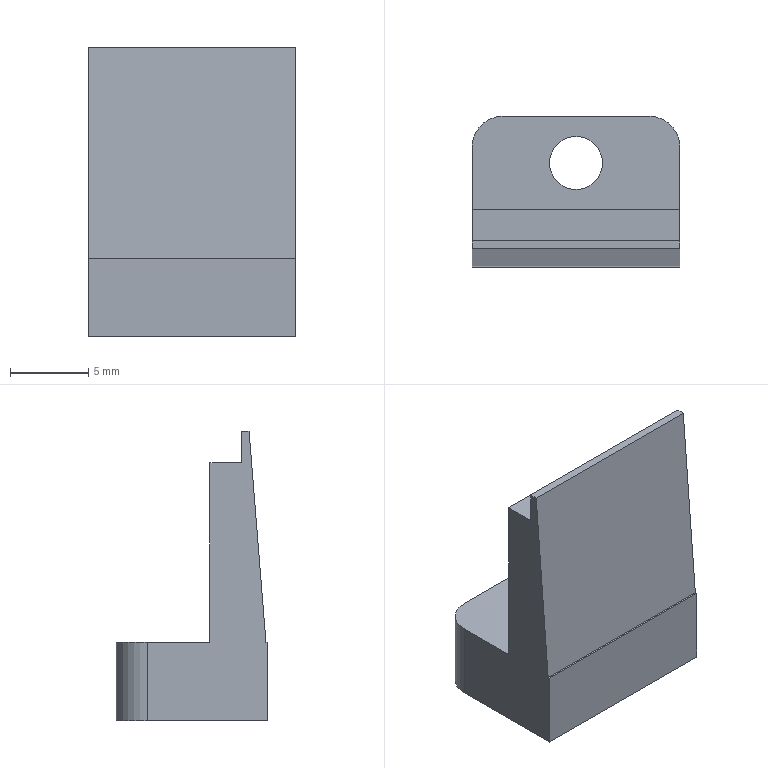Part | STEP file | 07-07 light-blocking plate | 1 solid | 20 faces | box 13.3 x 9.7 x 18.5 mm | volume 1003 mm3 | plane 13 | cylinder 7 | commonest cylinder face diameters 6.5 x3 3.4 x2 4 x2
STEP:
#1=CARTESIAN_POINT('',(3.25,4.85,3.4));
#2=VERTEX_POINT('',#1);
#3=CARTESIAN_POINT('',(-3.25,4.85,3.4));
#4=VERTEX_POINT('',#3);
#5=CARTESIAN_POINT('',(0.,4.85,3.4));
#6=DIRECTION('',(0.,0.,-1.));
#7=DIRECTION('',(-1.,0.,0.));
#8=AXIS2_PLACEMENT_3D('',#5,#6,#7);
#9=CIRCLE('',#8,3.25);
#10=EDGE_CURVE('',#2,#4,#9,.T.);
#11=ORIENTED_EDGE('',*,*,#10,.F.);
#12=CARTESIAN_POINT('',(3.25,4.85,0.));
#13=VERTEX_POINT('',#12);
#14=CARTESIAN_POINT('',(3.25,4.85,0.));
#15=DIRECTION('',(0.,0.,-1.));
#16=VECTOR('',#15,1000.);
#17=LINE('',#14,#16);
#18=EDGE_CURVE('',#2,#13,#17,.T.);
#19=ORIENTED_EDGE('',*,*,#18,.T.);
#20=CARTESIAN_POINT('',(-3.25,4.85,0.));
#21=VERTEX_POINT('',#20);
#22=CARTESIAN_POINT('',(0.,4.85,0.));
#23=DIRECTION('',(0.,0.,-1.));
#24=DIRECTION('',(-1.,0.,0.));
#25=AXIS2_PLACEMENT_3D('',#22,#23,#24);
#26=CIRCLE('',#25,3.25);
#27=EDGE_CURVE('',#13,#21,#26,.T.);
#28=ORIENTED_EDGE('',*,*,#27,.T.);
#29=CARTESIAN_POINT('',(-3.25,4.85,0.));
#30=DIRECTION('',(0.,0.,-1.));
#31=VECTOR('',#30,1000.);
#32=LINE('',#29,#31);
#33=EDGE_CURVE('',#4,#21,#32,.T.);
#34=ORIENTED_EDGE('',*,*,#33,.F.);
#35=EDGE_LOOP('',(#11,#19,#28,#34));
#36=FACE_OUTER_BOUND('',#35,.T.);
#37=CARTESIAN_POINT('',(0.,4.85,0.));
#38=DIRECTION('',(0.,0.,-1.));
#39=DIRECTION('',(-1.,0.,0.));
#40=AXIS2_PLACEMENT_3D('',#37,#38,#39);
#41=CYLINDRICAL_SURFACE('',#40,3.25);
#42=ADVANCED_FACE('',(#36),#41,.F.);
#43=CARTESIAN_POINT('',(-1.25,7.85,3.4));
#44=VERTEX_POINT('',#43);
#45=CARTESIAN_POINT('',(0.,4.85,3.4));
#46=DIRECTION('',(0.,0.,-1.));
#47=DIRECTION('',(-1.,0.,0.));
#48=AXIS2_PLACEMENT_3D('',#45,#46,#47);
#49=CIRCLE('',#48,3.25);
#50=EDGE_CURVE('',#4,#44,#49,.T.);
#51=ORIENTED_EDGE('',*,*,#50,.F.);
#52=ORIENTED_EDGE('',*,*,#33,.T.);
#53=CARTESIAN_POINT('',(-1.25,7.85,0.));
#54=VERTEX_POINT('',#53);
#55=CARTESIAN_POINT('',(0.,4.85,0.));
#56=DIRECTION('',(0.,0.,-1.));
#57=DIRECTION('',(-1.,0.,0.));
#58=AXIS2_PLACEMENT_3D('',#55,#56,#57);
#59=CIRCLE('',#58,3.25);
#60=EDGE_CURVE('',#21,#54,#59,.T.);
#61=ORIENTED_EDGE('',*,*,#60,.T.);
#62=CARTESIAN_POINT('',(-1.25,7.85,0.));
#63=DIRECTION('',(0.,0.,1.));
#64=VECTOR('',#63,1000.);
#65=LINE('',#62,#64);
#66=EDGE_CURVE('',#54,#44,#65,.T.);
#67=ORIENTED_EDGE('',*,*,#66,.T.);
#68=EDGE_LOOP('',(#51,#52,#61,#67));
#69=FACE_OUTER_BOUND('',#68,.T.);
#70=CARTESIAN_POINT('',(0.,4.85,0.));
#71=DIRECTION('',(0.,0.,-1.));
#72=DIRECTION('',(-1.,0.,0.));
#73=AXIS2_PLACEMENT_3D('',#70,#71,#72);
#74=CYLINDRICAL_SURFACE('',#73,3.25);
#75=ADVANCED_FACE('',(#69),#74,.F.);
#76=CARTESIAN_POINT('',(1.7,4.85,5.));
#77=VERTEX_POINT('',#76);
#78=CARTESIAN_POINT('',(-1.7,4.85,5.));
#79=VERTEX_POINT('',#78);
#80=CARTESIAN_POINT('',(0.,4.85,5.));
#81=DIRECTION('',(0.,0.,-1.));
#82=DIRECTION('',(-1.,0.,0.));
#83=AXIS2_PLACEMENT_3D('',#80,#81,#82);
#84=CIRCLE('',#83,1.7);
#85=EDGE_CURVE('',#77,#79,#84,.T.);
#86=ORIENTED_EDGE('',*,*,#85,.F.);
#87=CARTESIAN_POINT('',(1.7,4.85,3.4));
#88=VERTEX_POINT('',#87);
#89=CARTESIAN_POINT('',(1.7,4.85,0.));
#90=DIRECTION('',(0.,0.,-1.));
#91=VECTOR('',#90,1000.);
#92=LINE('',#89,#91);
#93=EDGE_CURVE('',#77,#88,#92,.T.);
#94=ORIENTED_EDGE('',*,*,#93,.T.);
#95=CARTESIAN_POINT('',(-1.7,4.85,3.4));
#96=VERTEX_POINT('',#95);
#97=CARTESIAN_POINT('',(0.,4.85,3.4));
#98=DIRECTION('',(0.,0.,-1.));
#99=DIRECTION('',(-1.,0.,0.));
#100=AXIS2_PLACEMENT_3D('',#97,#98,#99);
#101=CIRCLE('',#100,1.7);
#102=EDGE_CURVE('',#88,#96,#101,.T.);
#103=ORIENTED_EDGE('',*,*,#102,.T.);
#104=CARTESIAN_POINT('',(-1.7,4.85,0.));
#105=DIRECTION('',(0.,0.,-1.));
#106=VECTOR('',#105,1000.);
#107=LINE('',#104,#106);
#108=EDGE_CURVE('',#79,#96,#107,.T.);
#109=ORIENTED_EDGE('',*,*,#108,.F.);
#110=EDGE_LOOP('',(#86,#94,#103,#109));
#111=FACE_OUTER_BOUND('',#110,.T.);
#112=CARTESIAN_POINT('',(0.,4.85,0.));
#113=DIRECTION('',(0.,0.,-1.));
#114=DIRECTION('',(-1.,0.,0.));
#115=AXIS2_PLACEMENT_3D('',#112,#113,#114);
#116=CYLINDRICAL_SURFACE('',#115,1.7);
#117=ADVANCED_FACE('',(#111),#116,.F.);
#118=CARTESIAN_POINT('',(-6.65,1.85,5.));
#119=VERTEX_POINT('',#118);
#120=CARTESIAN_POINT('',(6.65,1.85,5.));
#121=VERTEX_POINT('',#120);
#122=CARTESIAN_POINT('',(-6.65,1.85,5.));
#123=DIRECTION('',(1.,0.,0.));
#124=VECTOR('',#123,1000.);
#125=LINE('',#122,#124);
#126=EDGE_CURVE('',#119,#121,#125,.T.);
#127=ORIENTED_EDGE('',*,*,#126,.F.);
#128=CARTESIAN_POINT('',(-6.65,1.85,16.5));
#129=VERTEX_POINT('',#128);
#130=CARTESIAN_POINT('',(-6.65,1.85,18.5));
#131=DIRECTION('',(0.,0.,-1.));
#132=VECTOR('',#131,1000.);
#133=LINE('',#130,#132);
#134=EDGE_CURVE('',#129,#119,#133,.T.);
#135=ORIENTED_EDGE('',*,*,#134,.F.);
#136=CARTESIAN_POINT('',(6.65,1.85,16.5));
#137=VERTEX_POINT('',#136);
#138=CARTESIAN_POINT('',(-6.65,1.85,16.5));
#139=DIRECTION('',(-1.,0.,0.));
#140=VECTOR('',#139,1000.);
#141=LINE('',#138,#140);
#142=EDGE_CURVE('',#137,#129,#141,.T.);
#143=ORIENTED_EDGE('',*,*,#142,.F.);
#144=CARTESIAN_POINT('',(6.65,1.85,18.5));
#145=DIRECTION('',(0.,0.,-1.));
#146=VECTOR('',#145,1000.);
#147=LINE('',#144,#146);
#148=EDGE_CURVE('',#137,#121,#147,.T.);
#149=ORIENTED_EDGE('',*,*,#148,.T.);
#150=EDGE_LOOP('',(#127,#135,#143,#149));
#151=FACE_OUTER_BOUND('',#150,.T.);
#152=CARTESIAN_POINT('',(-6.65,1.85,18.5));
#153=DIRECTION('',(0.,-1.,0.));
#154=DIRECTION('',(0.,0.,-1.));
#155=AXIS2_PLACEMENT_3D('',#152,#153,#154);
#156=PLANE('',#155);
#157=ADVANCED_FACE('',(#151),#156,.F.);
#158=CARTESIAN_POINT('',(-6.65,-1.73,5.));
#159=VERTEX_POINT('',#158);
#160=CARTESIAN_POINT('',(-6.65,-0.65,18.5));
#161=VERTEX_POINT('',#160);
#162=CARTESIAN_POINT('',(-6.65,-0.65,18.5));
#163=DIRECTION('',(0.,0.07975,0.9968));
#164=VECTOR('',#163,1000.);
#165=LINE('',#162,#164);
#166=EDGE_CURVE('',#159,#161,#165,.T.);
#167=ORIENTED_EDGE('',*,*,#166,.F.);
#168=CARTESIAN_POINT('',(6.65,-1.73,5.));
#169=VERTEX_POINT('',#168);
#170=CARTESIAN_POINT('',(6.65,-1.73,5.));
#171=DIRECTION('',(1.,0.,0.));
#172=VECTOR('',#171,1000.);
#173=LINE('',#170,#172);
#174=EDGE_CURVE('',#159,#169,#173,.T.);
#175=ORIENTED_EDGE('',*,*,#174,.T.);
#176=CARTESIAN_POINT('',(6.65,-0.65,18.5));
#177=VERTEX_POINT('',#176);
#178=CARTESIAN_POINT('',(6.65,-0.65,18.5));
#179=DIRECTION('',(0.,-0.07975,-0.9968));
#180=VECTOR('',#179,1000.);
#181=LINE('',#178,#180);
#182=EDGE_CURVE('',#177,#169,#181,.T.);
#183=ORIENTED_EDGE('',*,*,#182,.F.);
#184=CARTESIAN_POINT('',(6.65,-0.65,18.5));
#185=DIRECTION('',(1.,0.,0.));
#186=VECTOR('',#185,1000.);
#187=LINE('',#184,#186);
#188=EDGE_CURVE('',#161,#177,#187,.T.);
#189=ORIENTED_EDGE('',*,*,#188,.F.);
#190=EDGE_LOOP('',(#167,#175,#183,#189));
#191=FACE_OUTER_BOUND('',#190,.T.);
#192=CARTESIAN_POINT('',(6.65,-0.65,18.5));
#193=DIRECTION('',(0.,-0.9968,0.07975));
#194=DIRECTION('',(0.,-0.07975,-0.9968));
#195=AXIS2_PLACEMENT_3D('',#192,#193,#194);
#196=PLANE('',#195);
#197=ADVANCED_FACE('',(#191),#196,.T.);
#198=CARTESIAN_POINT('',(6.65,-1.85,0.));
#199=VERTEX_POINT('',#198);
#200=CARTESIAN_POINT('',(6.65,5.85,0.));
#201=VERTEX_POINT('',#200);
#202=CARTESIAN_POINT('',(6.65,1.85,0.));
#203=DIRECTION('',(0.,1.,0.));
#204=VECTOR('',#203,1000.);
#205=LINE('',#202,#204);
#206=EDGE_CURVE('',#199,#201,#205,.T.);
#207=ORIENTED_EDGE('',*,*,#206,.T.);
#208=CARTESIAN_POINT('',(6.65,5.85,5.));
#209=VERTEX_POINT('',#208);
#210=CARTESIAN_POINT('',(6.65,5.85,5.));
#211=DIRECTION('',(0.,0.,1.));
#212=VECTOR('',#211,1000.);
#213=LINE('',#210,#212);
#214=EDGE_CURVE('',#201,#209,#213,.T.);
#215=ORIENTED_EDGE('',*,*,#214,.T.);
#216=CARTESIAN_POINT('',(6.65,-1.85,5.));
#217=DIRECTION('',(0.,-1.,0.));
#218=VECTOR('',#217,1000.);
#219=LINE('',#216,#218);
#220=EDGE_CURVE('',#209,#121,#219,.T.);
#221=ORIENTED_EDGE('',*,*,#220,.T.);
#222=ORIENTED_EDGE('',*,*,#148,.F.);
#223=CARTESIAN_POINT('',(6.65,-0.15,16.5));
#224=VERTEX_POINT('',#223);
#225=CARTESIAN_POINT('',(6.65,1.85,16.5));
#226=DIRECTION('',(0.,1.,0.));
#227=VECTOR('',#226,1000.);
#228=LINE('',#225,#227);
#229=EDGE_CURVE('',#224,#137,#228,.T.);
#230=ORIENTED_EDGE('',*,*,#229,.F.);
#231=CARTESIAN_POINT('',(6.65,-0.15,18.5));
#232=VERTEX_POINT('',#231);
#233=CARTESIAN_POINT('',(6.65,-0.15,16.5));
#234=DIRECTION('',(0.,0.,1.));
#235=VECTOR('',#234,1000.);
#236=LINE('',#233,#235);
#237=EDGE_CURVE('',#224,#232,#236,.T.);
#238=ORIENTED_EDGE('',*,*,#237,.T.);
#239=CARTESIAN_POINT('',(6.65,1.85,18.5));
#240=DIRECTION('',(0.,1.,0.));
#241=VECTOR('',#240,1000.);
#242=LINE('',#239,#241);
#243=EDGE_CURVE('',#177,#232,#242,.T.);
#244=ORIENTED_EDGE('',*,*,#243,.F.);
#245=ORIENTED_EDGE('',*,*,#182,.T.);
#246=CARTESIAN_POINT('',(6.65,-1.85,5.));
#247=VERTEX_POINT('',#246);
#248=CARTESIAN_POINT('',(6.65,-1.85,5.));
#249=DIRECTION('',(0.,-1.,0.));
#250=VECTOR('',#249,1000.);
#251=LINE('',#248,#250);
#252=EDGE_CURVE('',#169,#247,#251,.T.);
#253=ORIENTED_EDGE('',*,*,#252,.T.);
#254=CARTESIAN_POINT('',(6.65,-1.85,18.5));
#255=DIRECTION('',(0.,0.,-1.));
#256=VECTOR('',#255,1000.);
#257=LINE('',#254,#256);
#258=EDGE_CURVE('',#247,#199,#257,.T.);
#259=ORIENTED_EDGE('',*,*,#258,.T.);
#260=EDGE_LOOP('',(#207,#215,#221,#222,#230,#238,#244,#245,#253,#259));
#261=FACE_OUTER_BOUND('',#260,.T.);
#262=CARTESIAN_POINT('',(6.65,1.85,18.5));
#263=DIRECTION('',(-1.,0.,0.));
#264=DIRECTION('',(0.,-1.,0.));
#265=AXIS2_PLACEMENT_3D('',#262,#263,#264);
#266=PLANE('',#265);
#267=ADVANCED_FACE('',(#261),#266,.F.);
#268=CARTESIAN_POINT('',(-6.65,5.85,5.));
#269=VERTEX_POINT('',#268);
#270=CARTESIAN_POINT('',(-6.65,-1.85,5.));
#271=DIRECTION('',(0.,1.,0.));
#272=VECTOR('',#271,1000.);
#273=LINE('',#270,#272);
#274=EDGE_CURVE('',#119,#269,#273,.T.);
#275=ORIENTED_EDGE('',*,*,#274,.T.);
#276=CARTESIAN_POINT('',(-6.65,5.85,0.));
#277=VERTEX_POINT('',#276);
#278=CARTESIAN_POINT('',(-6.65,5.85,0.));
#279=DIRECTION('',(0.,0.,-1.));
#280=VECTOR('',#279,1000.);
#281=LINE('',#278,#280);
#282=EDGE_CURVE('',#269,#277,#281,.T.);
#283=ORIENTED_EDGE('',*,*,#282,.T.);
#284=CARTESIAN_POINT('',(-6.65,-1.85,0.));
#285=VERTEX_POINT('',#284);
#286=CARTESIAN_POINT('',(-6.65,1.85,0.));
#287=DIRECTION('',(0.,-1.,0.));
#288=VECTOR('',#287,1000.);
#289=LINE('',#286,#288);
#290=EDGE_CURVE('',#277,#285,#289,.T.);
#291=ORIENTED_EDGE('',*,*,#290,.T.);
#292=CARTESIAN_POINT('',(-6.65,-1.85,5.));
#293=VERTEX_POINT('',#292);
#294=CARTESIAN_POINT('',(-6.65,-1.85,18.5));
#295=DIRECTION('',(0.,0.,-1.));
#296=VECTOR('',#295,1000.);
#297=LINE('',#294,#296);
#298=EDGE_CURVE('',#293,#285,#297,.T.);
#299=ORIENTED_EDGE('',*,*,#298,.F.);
#300=CARTESIAN_POINT('',(-6.65,-1.85,5.));
#301=DIRECTION('',(0.,1.,0.));
#302=VECTOR('',#301,1000.);
#303=LINE('',#300,#302);
#304=EDGE_CURVE('',#293,#159,#303,.T.);
#305=ORIENTED_EDGE('',*,*,#304,.T.);
#306=ORIENTED_EDGE('',*,*,#166,.T.);
#307=CARTESIAN_POINT('',(-6.65,-0.15,18.5));
#308=VERTEX_POINT('',#307);
#309=CARTESIAN_POINT('',(-6.65,1.85,18.5));
#310=DIRECTION('',(0.,-1.,0.));
#311=VECTOR('',#310,1000.);
#312=LINE('',#309,#311);
#313=EDGE_CURVE('',#308,#161,#312,.T.);
#314=ORIENTED_EDGE('',*,*,#313,.F.);
#315=CARTESIAN_POINT('',(-6.65,-0.15,16.5));
#316=VERTEX_POINT('',#315);
#317=CARTESIAN_POINT('',(-6.65,-0.15,16.5));
#318=DIRECTION('',(0.,0.,1.));
#319=VECTOR('',#318,1000.);
#320=LINE('',#317,#319);
#321=EDGE_CURVE('',#316,#308,#320,.T.);
#322=ORIENTED_EDGE('',*,*,#321,.F.);
#323=CARTESIAN_POINT('',(-6.65,1.85,16.5));
#324=DIRECTION('',(0.,-1.,0.));
#325=VECTOR('',#324,1000.);
#326=LINE('',#323,#325);
#327=EDGE_CURVE('',#129,#316,#326,.T.);
#328=ORIENTED_EDGE('',*,*,#327,.F.);
#329=ORIENTED_EDGE('',*,*,#134,.T.);
#330=EDGE_LOOP('',(#275,#283,#291,#299,#305,#306,#314,#322,#328,#329));
#331=FACE_OUTER_BOUND('',#330,.T.);
#332=CARTESIAN_POINT('',(-6.65,1.85,18.5));
#333=DIRECTION('',(1.,0.,0.));
#334=DIRECTION('',(0.,1.,0.));
#335=AXIS2_PLACEMENT_3D('',#332,#333,#334);
#336=PLANE('',#335);
#337=ADVANCED_FACE('',(#331),#336,.F.);
#338=ORIENTED_EDGE('',*,*,#258,.F.);
#339=CARTESIAN_POINT('',(-6.65,-1.85,5.));
#340=DIRECTION('',(-1.,0.,0.));
#341=VECTOR('',#340,1000.);
#342=LINE('',#339,#341);
#343=EDGE_CURVE('',#247,#293,#342,.T.);
#344=ORIENTED_EDGE('',*,*,#343,.T.);
#345=ORIENTED_EDGE('',*,*,#298,.T.);
#346=CARTESIAN_POINT('',(-6.65,-1.85,0.));
#347=DIRECTION('',(1.,0.,0.));
#348=VECTOR('',#347,1000.);
#349=LINE('',#346,#348);
#350=EDGE_CURVE('',#285,#199,#349,.T.);
#351=ORIENTED_EDGE('',*,*,#350,.T.);
#352=EDGE_LOOP('',(#338,#344,#345,#351));
#353=FACE_OUTER_BOUND('',#352,.T.);
#354=CARTESIAN_POINT('',(-6.65,-1.85,18.5));
#355=DIRECTION('',(0.,1.,0.));
#356=DIRECTION('',(0.,0.,1.));
#357=AXIS2_PLACEMENT_3D('',#354,#355,#356);
#358=PLANE('',#357);
#359=ADVANCED_FACE('',(#353),#358,.F.);
#360=ORIENTED_EDGE('',*,*,#313,.T.);
#361=ORIENTED_EDGE('',*,*,#188,.T.);
#362=ORIENTED_EDGE('',*,*,#243,.T.);
#363=CARTESIAN_POINT('',(-6.65,-0.15,18.5));
#364=DIRECTION('',(1.,0.,0.));
#365=VECTOR('',#364,1000.);
#366=LINE('',#363,#365);
#367=EDGE_CURVE('',#308,#232,#366,.T.);
#368=ORIENTED_EDGE('',*,*,#367,.F.);
#369=EDGE_LOOP('',(#360,#361,#362,#368));
#370=FACE_OUTER_BOUND('',#369,.T.);
#371=CARTESIAN_POINT('',(6.65,-1.85,18.5));
#372=DIRECTION('',(0.,0.,1.));
#373=DIRECTION('',(1.,0.,0.));
#374=AXIS2_PLACEMENT_3D('',#371,#372,#373);
#375=PLANE('',#374);
#376=ADVANCED_FACE('',(#370),#375,.T.);
#377=CARTESIAN_POINT('',(-4.65,7.85,0.));
#378=VERTEX_POINT('',#377);
#379=CARTESIAN_POINT('',(-6.65,7.85,0.));
#380=DIRECTION('',(1.,0.,0.));
#381=VECTOR('',#380,1000.);
#382=LINE('',#379,#381);
#383=EDGE_CURVE('',#378,#54,#382,.T.);
#384=ORIENTED_EDGE('',*,*,#383,.T.);
#385=ORIENTED_EDGE('',*,*,#60,.F.);
#386=ORIENTED_EDGE('',*,*,#27,.F.);
#387=CARTESIAN_POINT('',(1.25,7.85,0.));
#388=VERTEX_POINT('',#387);
#389=CARTESIAN_POINT('',(0.,4.85,0.));
#390=DIRECTION('',(0.,0.,-1.));
#391=DIRECTION('',(-1.,0.,0.));
#392=AXIS2_PLACEMENT_3D('',#389,#390,#391);
#393=CIRCLE('',#392,3.25);
#394=EDGE_CURVE('',#388,#13,#393,.T.);
#395=ORIENTED_EDGE('',*,*,#394,.F.);
#396=CARTESIAN_POINT('',(4.65,7.85,0.));
#397=VERTEX_POINT('',#396);
#398=CARTESIAN_POINT('',(-6.65,7.85,0.));
#399=DIRECTION('',(1.,0.,0.));
#400=VECTOR('',#399,1000.);
#401=LINE('',#398,#400);
#402=EDGE_CURVE('',#388,#397,#401,.T.);
#403=ORIENTED_EDGE('',*,*,#402,.T.);
#404=CARTESIAN_POINT('',(4.65,5.85,0.));
#405=DIRECTION('',(0.,0.,-1.));
#406=DIRECTION('',(1.,0.,0.));
#407=AXIS2_PLACEMENT_3D('',#404,#405,#406);
#408=CIRCLE('',#407,2.);
#409=EDGE_CURVE('',#397,#201,#408,.T.);
#410=ORIENTED_EDGE('',*,*,#409,.T.);
#411=ORIENTED_EDGE('',*,*,#206,.F.);
#412=ORIENTED_EDGE('',*,*,#350,.F.);
#413=ORIENTED_EDGE('',*,*,#290,.F.);
#414=CARTESIAN_POINT('',(-4.65,5.85,0.));
#415=DIRECTION('',(0.,0.,-1.));
#416=DIRECTION('',(1.,0.,0.));
#417=AXIS2_PLACEMENT_3D('',#414,#415,#416);
#418=CIRCLE('',#417,2.);
#419=EDGE_CURVE('',#277,#378,#418,.T.);
#420=ORIENTED_EDGE('',*,*,#419,.T.);
#421=EDGE_LOOP('',(#384,#385,#386,#395,#403,#410,#411,#412,#413,#420));
#422=FACE_OUTER_BOUND('',#421,.T.);
#423=CARTESIAN_POINT('',(6.65,-1.85,0.));
#424=DIRECTION('',(0.,0.,1.));
#425=DIRECTION('',(1.,0.,0.));
#426=AXIS2_PLACEMENT_3D('',#423,#424,#425);
#427=PLANE('',#426);
#428=ADVANCED_FACE('',(#422),#427,.F.);
#429=ORIENTED_EDGE('',*,*,#367,.T.);
#430=ORIENTED_EDGE('',*,*,#237,.F.);
#431=CARTESIAN_POINT('',(-6.65,-0.15,16.5));
#432=DIRECTION('',(1.,0.,0.));
#433=VECTOR('',#432,1000.);
#434=LINE('',#431,#433);
#435=EDGE_CURVE('',#316,#224,#434,.T.);
#436=ORIENTED_EDGE('',*,*,#435,.F.);
#437=ORIENTED_EDGE('',*,*,#321,.T.);
#438=EDGE_LOOP('',(#429,#430,#436,#437));
#439=FACE_OUTER_BOUND('',#438,.T.);
#440=CARTESIAN_POINT('',(-6.65,-0.15,16.5));
#441=DIRECTION('',(0.,-1.,0.));
#442=DIRECTION('',(0.,0.,-1.));
#443=AXIS2_PLACEMENT_3D('',#440,#441,#442);
#444=PLANE('',#443);
#445=ADVANCED_FACE('',(#439),#444,.F.);
#446=ORIENTED_EDGE('',*,*,#327,.T.);
#447=ORIENTED_EDGE('',*,*,#435,.T.);
#448=ORIENTED_EDGE('',*,*,#229,.T.);
#449=ORIENTED_EDGE('',*,*,#142,.T.);
#450=EDGE_LOOP('',(#446,#447,#448,#449));
#451=FACE_OUTER_BOUND('',#450,.T.);
#452=CARTESIAN_POINT('',(-6.65,-0.15,16.5));
#453=DIRECTION('',(0.,0.,1.));
#454=DIRECTION('',(1.,0.,0.));
#455=AXIS2_PLACEMENT_3D('',#452,#453,#454);
#456=PLANE('',#455);
#457=ADVANCED_FACE('',(#451),#456,.T.);
#458=ORIENTED_EDGE('',*,*,#174,.F.);
#459=ORIENTED_EDGE('',*,*,#304,.F.);
#460=ORIENTED_EDGE('',*,*,#343,.F.);
#461=ORIENTED_EDGE('',*,*,#252,.F.);
#462=EDGE_LOOP('',(#458,#459,#460,#461));
#463=FACE_OUTER_BOUND('',#462,.T.);
#464=CARTESIAN_POINT('',(-6.65,7.85,5.));
#465=DIRECTION('',(0.,0.,-1.));
#466=DIRECTION('',(-1.,0.,0.));
#467=AXIS2_PLACEMENT_3D('',#464,#465,#466);
#468=PLANE('',#467);
#469=ADVANCED_FACE('',(#463),#468,.F.);
#470=CARTESIAN_POINT('',(0.,4.85,5.));
#471=DIRECTION('',(0.,0.,-1.));
#472=DIRECTION('',(-1.,0.,0.));
#473=AXIS2_PLACEMENT_3D('',#470,#471,#472);
#474=CIRCLE('',#473,1.7);
#475=EDGE_CURVE('',#79,#77,#474,.T.);
#476=ORIENTED_EDGE('',*,*,#475,.T.);
#477=ORIENTED_EDGE('',*,*,#85,.T.);
#478=EDGE_LOOP('',(#476,#477));
#479=FACE_BOUND('',#478,.T.);
#480=ORIENTED_EDGE('',*,*,#220,.F.);
#481=CARTESIAN_POINT('',(4.65,7.85,5.));
#482=VERTEX_POINT('',#481);
#483=CARTESIAN_POINT('',(4.65,5.85,5.));
#484=DIRECTION('',(0.,0.,1.));
#485=DIRECTION('',(-1.,0.,0.));
#486=AXIS2_PLACEMENT_3D('',#483,#484,#485);
#487=CIRCLE('',#486,2.);
#488=EDGE_CURVE('',#209,#482,#487,.T.);
#489=ORIENTED_EDGE('',*,*,#488,.T.);
#490=CARTESIAN_POINT('',(-4.65,7.85,5.));
#491=VERTEX_POINT('',#490);
#492=CARTESIAN_POINT('',(-6.65,7.85,5.));
#493=DIRECTION('',(1.,0.,0.));
#494=VECTOR('',#493,1000.);
#495=LINE('',#492,#494);
#496=EDGE_CURVE('',#491,#482,#495,.T.);
#497=ORIENTED_EDGE('',*,*,#496,.F.);
#498=CARTESIAN_POINT('',(-4.65,5.85,5.));
#499=DIRECTION('',(0.,0.,1.));
#500=DIRECTION('',(-1.,0.,0.));
#501=AXIS2_PLACEMENT_3D('',#498,#499,#500);
#502=CIRCLE('',#501,2.);
#503=EDGE_CURVE('',#491,#269,#502,.T.);
#504=ORIENTED_EDGE('',*,*,#503,.T.);
#505=ORIENTED_EDGE('',*,*,#274,.F.);
#506=ORIENTED_EDGE('',*,*,#126,.T.);
#507=EDGE_LOOP('',(#480,#489,#497,#504,#505,#506));
#508=FACE_OUTER_BOUND('',#507,.T.);
#509=CARTESIAN_POINT('',(-6.65,7.85,5.));
#510=DIRECTION('',(0.,0.,-1.));
#511=DIRECTION('',(-1.,0.,0.));
#512=AXIS2_PLACEMENT_3D('',#509,#510,#511);
#513=PLANE('',#512);
#514=ADVANCED_FACE('',(#479,#508),#513,.F.);
#515=CARTESIAN_POINT('',(1.25,7.85,3.4));
#516=VERTEX_POINT('',#515);
#517=CARTESIAN_POINT('',(1.25,7.85,0.));
#518=DIRECTION('',(0.,0.,-1.));
#519=VECTOR('',#518,1000.);
#520=LINE('',#517,#519);
#521=EDGE_CURVE('',#516,#388,#520,.T.);
#522=ORIENTED_EDGE('',*,*,#521,.F.);
#523=CARTESIAN_POINT('',(-6.65,7.85,3.4));
#524=DIRECTION('',(1.,0.,0.));
#525=VECTOR('',#524,1000.);
#526=LINE('',#523,#525);
#527=EDGE_CURVE('',#44,#516,#526,.T.);
#528=ORIENTED_EDGE('',*,*,#527,.F.);
#529=ORIENTED_EDGE('',*,*,#66,.F.);
#530=ORIENTED_EDGE('',*,*,#383,.F.);
#531=CARTESIAN_POINT('',(-4.65,7.85,5.));
#532=DIRECTION('',(0.,0.,1.));
#533=VECTOR('',#532,1000.);
#534=LINE('',#531,#533);
#535=EDGE_CURVE('',#378,#491,#534,.T.);
#536=ORIENTED_EDGE('',*,*,#535,.T.);
#537=ORIENTED_EDGE('',*,*,#496,.T.);
#538=CARTESIAN_POINT('',(4.65,7.85,0.));
#539=DIRECTION('',(0.,0.,-1.));
#540=VECTOR('',#539,1000.);
#541=LINE('',#538,#540);
#542=EDGE_CURVE('',#482,#397,#541,.T.);
#543=ORIENTED_EDGE('',*,*,#542,.T.);
#544=ORIENTED_EDGE('',*,*,#402,.F.);
#545=EDGE_LOOP('',(#522,#528,#529,#530,#536,#537,#543,#544));
#546=FACE_OUTER_BOUND('',#545,.T.);
#547=CARTESIAN_POINT('',(-6.65,7.85,5.));
#548=DIRECTION('',(0.,1.,0.));
#549=DIRECTION('',(-1.,0.,0.));
#550=AXIS2_PLACEMENT_3D('',#547,#548,#549);
#551=PLANE('',#550);
#552=ADVANCED_FACE('',(#546),#551,.T.);
#553=ORIENTED_EDGE('',*,*,#488,.F.);
#554=ORIENTED_EDGE('',*,*,#214,.F.);
#555=ORIENTED_EDGE('',*,*,#409,.F.);
#556=ORIENTED_EDGE('',*,*,#542,.F.);
#557=EDGE_LOOP('',(#553,#554,#555,#556));
#558=FACE_OUTER_BOUND('',#557,.T.);
#559=CARTESIAN_POINT('',(4.65,5.85,5.));
#560=DIRECTION('',(0.,0.,1.));
#561=DIRECTION('',(1.,0.,0.));
#562=AXIS2_PLACEMENT_3D('',#559,#560,#561);
#563=CYLINDRICAL_SURFACE('',#562,2.);
#564=ADVANCED_FACE('',(#558),#563,.T.);
#565=ORIENTED_EDGE('',*,*,#503,.F.);
#566=ORIENTED_EDGE('',*,*,#535,.F.);
#567=ORIENTED_EDGE('',*,*,#419,.F.);
#568=ORIENTED_EDGE('',*,*,#282,.F.);
#569=EDGE_LOOP('',(#565,#566,#567,#568));
#570=FACE_OUTER_BOUND('',#569,.T.);
#571=CARTESIAN_POINT('',(-4.65,5.85,18.5));
#572=DIRECTION('',(0.,0.,1.));
#573=DIRECTION('',(1.,0.,0.));
#574=AXIS2_PLACEMENT_3D('',#571,#572,#573);
#575=CYLINDRICAL_SURFACE('',#574,2.);
#576=ADVANCED_FACE('',(#570),#575,.T.);
#577=ORIENTED_EDGE('',*,*,#93,.F.);
#578=ORIENTED_EDGE('',*,*,#475,.F.);
#579=ORIENTED_EDGE('',*,*,#108,.T.);
#580=CARTESIAN_POINT('',(0.,4.85,3.4));
#581=DIRECTION('',(0.,0.,-1.));
#582=DIRECTION('',(-1.,0.,0.));
#583=AXIS2_PLACEMENT_3D('',#580,#581,#582);
#584=CIRCLE('',#583,1.7);
#585=EDGE_CURVE('',#96,#88,#584,.T.);
#586=ORIENTED_EDGE('',*,*,#585,.T.);
#587=EDGE_LOOP('',(#577,#578,#579,#586));
#588=FACE_OUTER_BOUND('',#587,.T.);
#589=CARTESIAN_POINT('',(0.,4.85,0.));
#590=DIRECTION('',(0.,0.,-1.));
#591=DIRECTION('',(-1.,0.,0.));
#592=AXIS2_PLACEMENT_3D('',#589,#590,#591);
#593=CYLINDRICAL_SURFACE('',#592,1.7);
#594=ADVANCED_FACE('',(#588),#593,.F.);
#595=ORIENTED_EDGE('',*,*,#527,.T.);
#596=CARTESIAN_POINT('',(0.,4.85,3.4));
#597=DIRECTION('',(0.,0.,-1.));
#598=DIRECTION('',(-1.,0.,0.));
#599=AXIS2_PLACEMENT_3D('',#596,#597,#598);
#600=CIRCLE('',#599,3.25);
#601=EDGE_CURVE('',#516,#2,#600,.T.);
#602=ORIENTED_EDGE('',*,*,#601,.T.);
#603=ORIENTED_EDGE('',*,*,#10,.T.);
#604=ORIENTED_EDGE('',*,*,#50,.T.);
#605=EDGE_LOOP('',(#595,#602,#603,#604));
#606=FACE_OUTER_BOUND('',#605,.T.);
#607=ORIENTED_EDGE('',*,*,#585,.F.);
#608=ORIENTED_EDGE('',*,*,#102,.F.);
#609=EDGE_LOOP('',(#607,#608));
#610=FACE_BOUND('',#609,.T.);
#611=CARTESIAN_POINT('',(1.7,4.85,3.4));
#612=DIRECTION('',(0.,0.,1.));
#613=DIRECTION('',(1.,0.,0.));
#614=AXIS2_PLACEMENT_3D('',#611,#612,#613);
#615=PLANE('',#614);
#616=ADVANCED_FACE('',(#606,#610),#615,.F.);
#617=ORIENTED_EDGE('',*,*,#18,.F.);
#618=ORIENTED_EDGE('',*,*,#601,.F.);
#619=ORIENTED_EDGE('',*,*,#521,.T.);
#620=ORIENTED_EDGE('',*,*,#394,.T.);
#621=EDGE_LOOP('',(#617,#618,#619,#620));
#622=FACE_OUTER_BOUND('',#621,.T.);
#623=CARTESIAN_POINT('',(0.,4.85,0.));
#624=DIRECTION('',(0.,0.,-1.));
#625=DIRECTION('',(-1.,0.,0.));
#626=AXIS2_PLACEMENT_3D('',#623,#624,#625);
#627=CYLINDRICAL_SURFACE('',#626,3.25);
#628=ADVANCED_FACE('',(#622),#627,.F.);
#629=CLOSED_SHELL('',(#42,#75,#117,#157,#197,#267,#337,#359,#376,#428,#445,#457,#469,#514,#552,#564,#576,#594,#616,#628));
#630=MANIFOLD_SOLID_BREP('',#629);
#631=CARTESIAN_POINT('',(0.,0.,0.));
#632=DIRECTION('',(0.,0.,1.));
#633=DIRECTION('',(1.,0.,0.));
#634=AXIS2_PLACEMENT_3D('',#631,#632,#633);
#635=(LENGTH_UNIT()NAMED_UNIT(*)SI_UNIT(.MILLI.,.METRE.));
#636=UNCERTAINTY_MEASURE_WITH_UNIT(LENGTH_MEASURE(0.00001),#635,'','');
#637=(NAMED_UNIT(*)PLANE_ANGLE_UNIT()SI_UNIT($,.RADIAN.));
#638=(NAMED_UNIT(*)SI_UNIT($,.STERADIAN.)SOLID_ANGLE_UNIT());
#639=(GEOMETRIC_REPRESENTATION_CONTEXT(3)GLOBAL_UNCERTAINTY_ASSIGNED_CONTEXT((#636))GLOBAL_UNIT_ASSIGNED_CONTEXT((#635,#637,#638))REPRESENTATION_CONTEXT('',''));
#640=ADVANCED_BREP_SHAPE_REPRESENTATION('',(#630,#634),#639);